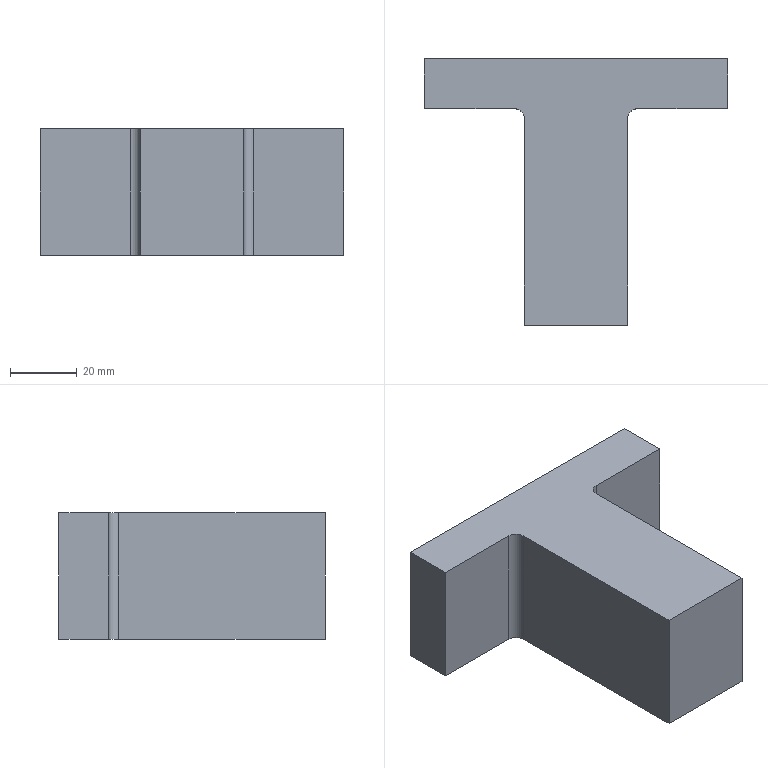Part | SolidWorks | features Extrusion 1, Fillet 1, ICE 1 | 1 solid | 12 faces | box 91 x 80 x 38 mm | volume 128587 mm3 | plane 10 | cylinder 2 | commonest cylinder face diameters 6 x2
STEP:
#1=CARTESIAN_POINT('',(45.5,25.,19.));
#2=VERTEX_POINT('',#1);
#3=CARTESIAN_POINT('',(45.5,40.,19.));
#4=VERTEX_POINT('',#3);
#5=CARTESIAN_POINT('',(45.5,-40.,19.));
#6=DIRECTION('',(0.,1.,0.));
#7=VECTOR('',#6,1000.);
#8=LINE('',#5,#7);
#9=EDGE_CURVE('',#2,#4,#8,.T.);
#10=ORIENTED_EDGE('',*,*,#9,.F.);
#11=CARTESIAN_POINT('',(45.5,25.,-19.));
#12=VERTEX_POINT('',#11);
#13=CARTESIAN_POINT('',(45.5,25.,-19.001));
#14=DIRECTION('',(0.,0.,1.));
#15=VECTOR('',#14,1000.);
#16=LINE('',#13,#15);
#17=EDGE_CURVE('',#12,#2,#16,.T.);
#18=ORIENTED_EDGE('',*,*,#17,.F.);
#19=CARTESIAN_POINT('',(45.5,40.,-19.));
#20=VERTEX_POINT('',#19);
#21=CARTESIAN_POINT('',(45.5,-40.,-19.));
#22=DIRECTION('',(0.,1.,0.));
#23=VECTOR('',#22,1000.);
#24=LINE('',#21,#23);
#25=EDGE_CURVE('',#12,#20,#24,.T.);
#26=ORIENTED_EDGE('',*,*,#25,.T.);
#27=CARTESIAN_POINT('',(45.5,40.,19.));
#28=DIRECTION('',(0.,0.,-1.));
#29=VECTOR('',#28,1000.);
#30=LINE('',#27,#29);
#31=EDGE_CURVE('',#4,#20,#30,.T.);
#32=ORIENTED_EDGE('',*,*,#31,.F.);
#33=EDGE_LOOP('',(#10,#18,#26,#32));
#34=FACE_OUTER_BOUND('',#33,.T.);
#35=CARTESIAN_POINT('',(45.5,-40.,19.));
#36=DIRECTION('',(-1.,0.,0.));
#37=DIRECTION('',(0.,0.,1.));
#38=AXIS2_PLACEMENT_3D('',#35,#36,#37);
#39=PLANE('',#38);
#40=ADVANCED_FACE('',(#34),#39,.F.);
#41=CARTESIAN_POINT('',(-45.5,40.,-19.));
#42=VERTEX_POINT('',#41);
#43=CARTESIAN_POINT('',(-45.5,40.,-19.));
#44=DIRECTION('',(-1.,0.,0.));
#45=VECTOR('',#44,1000.);
#46=LINE('',#43,#45);
#47=EDGE_CURVE('',#20,#42,#46,.T.);
#48=ORIENTED_EDGE('',*,*,#47,.T.);
#49=CARTESIAN_POINT('',(-45.5,40.,19.));
#50=VERTEX_POINT('',#49);
#51=CARTESIAN_POINT('',(-45.5,40.,19.));
#52=DIRECTION('',(0.,0.,-1.));
#53=VECTOR('',#52,1000.);
#54=LINE('',#51,#53);
#55=EDGE_CURVE('',#50,#42,#54,.T.);
#56=ORIENTED_EDGE('',*,*,#55,.F.);
#57=CARTESIAN_POINT('',(-45.5,40.,19.));
#58=DIRECTION('',(-1.,0.,0.));
#59=VECTOR('',#58,1000.);
#60=LINE('',#57,#59);
#61=EDGE_CURVE('',#4,#50,#60,.T.);
#62=ORIENTED_EDGE('',*,*,#61,.F.);
#63=ORIENTED_EDGE('',*,*,#31,.T.);
#64=EDGE_LOOP('',(#48,#56,#62,#63));
#65=FACE_OUTER_BOUND('',#64,.T.);
#66=CARTESIAN_POINT('',(-45.5,40.,19.));
#67=DIRECTION('',(0.,-1.,0.));
#68=DIRECTION('',(0.,0.,-1.));
#69=AXIS2_PLACEMENT_3D('',#66,#67,#68);
#70=PLANE('',#69);
#71=ADVANCED_FACE('',(#65),#70,.F.);
#72=CARTESIAN_POINT('',(-45.5,25.,-19.));
#73=VERTEX_POINT('',#72);
#74=CARTESIAN_POINT('',(-45.5,-40.,-19.));
#75=DIRECTION('',(0.,-1.,0.));
#76=VECTOR('',#75,1000.);
#77=LINE('',#74,#76);
#78=EDGE_CURVE('',#42,#73,#77,.T.);
#79=ORIENTED_EDGE('',*,*,#78,.T.);
#80=CARTESIAN_POINT('',(-45.5,25.,19.));
#81=VERTEX_POINT('',#80);
#82=CARTESIAN_POINT('',(-45.5,25.,-19.001));
#83=DIRECTION('',(0.,0.,1.));
#84=VECTOR('',#83,1000.);
#85=LINE('',#82,#84);
#86=EDGE_CURVE('',#73,#81,#85,.T.);
#87=ORIENTED_EDGE('',*,*,#86,.T.);
#88=CARTESIAN_POINT('',(-45.5,-40.,19.));
#89=DIRECTION('',(0.,-1.,0.));
#90=VECTOR('',#89,1000.);
#91=LINE('',#88,#90);
#92=EDGE_CURVE('',#50,#81,#91,.T.);
#93=ORIENTED_EDGE('',*,*,#92,.F.);
#94=ORIENTED_EDGE('',*,*,#55,.T.);
#95=EDGE_LOOP('',(#79,#87,#93,#94));
#96=FACE_OUTER_BOUND('',#95,.T.);
#97=CARTESIAN_POINT('',(-45.5,-40.,19.));
#98=DIRECTION('',(1.,0.,0.));
#99=DIRECTION('',(0.,0.,-1.));
#100=AXIS2_PLACEMENT_3D('',#97,#98,#99);
#101=PLANE('',#100);
#102=ADVANCED_FACE('',(#96),#101,.F.);
#103=CARTESIAN_POINT('',(-15.5,-40.,19.));
#104=VERTEX_POINT('',#103);
#105=CARTESIAN_POINT('',(15.5,-40.,19.));
#106=VERTEX_POINT('',#105);
#107=CARTESIAN_POINT('',(-45.5,-40.,19.));
#108=DIRECTION('',(1.,0.,0.));
#109=VECTOR('',#108,1000.);
#110=LINE('',#107,#109);
#111=EDGE_CURVE('',#104,#106,#110,.T.);
#112=ORIENTED_EDGE('',*,*,#111,.F.);
#113=CARTESIAN_POINT('',(-15.5,-40.,-19.));
#114=VERTEX_POINT('',#113);
#115=CARTESIAN_POINT('',(-15.5,-40.,-19.001));
#116=DIRECTION('',(0.,0.,1.));
#117=VECTOR('',#116,1000.);
#118=LINE('',#115,#117);
#119=EDGE_CURVE('',#114,#104,#118,.T.);
#120=ORIENTED_EDGE('',*,*,#119,.F.);
#121=CARTESIAN_POINT('',(15.5,-40.,-19.));
#122=VERTEX_POINT('',#121);
#123=CARTESIAN_POINT('',(-45.5,-40.,-19.));
#124=DIRECTION('',(1.,0.,0.));
#125=VECTOR('',#124,1000.);
#126=LINE('',#123,#125);
#127=EDGE_CURVE('',#114,#122,#126,.T.);
#128=ORIENTED_EDGE('',*,*,#127,.T.);
#129=CARTESIAN_POINT('',(15.5,-40.,-19.001));
#130=DIRECTION('',(0.,0.,1.));
#131=VECTOR('',#130,1000.);
#132=LINE('',#129,#131);
#133=EDGE_CURVE('',#122,#106,#132,.T.);
#134=ORIENTED_EDGE('',*,*,#133,.T.);
#135=EDGE_LOOP('',(#112,#120,#128,#134));
#136=FACE_OUTER_BOUND('',#135,.T.);
#137=CARTESIAN_POINT('',(-45.5,-40.,19.));
#138=DIRECTION('',(0.,1.,0.));
#139=DIRECTION('',(0.,0.,1.));
#140=AXIS2_PLACEMENT_3D('',#137,#138,#139);
#141=PLANE('',#140);
#142=ADVANCED_FACE('',(#136),#141,.F.);
#143=ORIENTED_EDGE('',*,*,#92,.T.);
#144=CARTESIAN_POINT('',(-18.5,25.,19.));
#145=VERTEX_POINT('',#144);
#146=CARTESIAN_POINT('',(-45.5,25.,19.));
#147=DIRECTION('',(-1.,0.,0.));
#148=VECTOR('',#147,1000.);
#149=LINE('',#146,#148);
#150=EDGE_CURVE('',#145,#81,#149,.T.);
#151=ORIENTED_EDGE('',*,*,#150,.F.);
#152=CARTESIAN_POINT('',(-15.5,22.,19.));
#153=VERTEX_POINT('',#152);
#154=CARTESIAN_POINT('',(-18.5,22.,19.));
#155=DIRECTION('',(0.,0.,-1.));
#156=DIRECTION('',(-1.,0.,0.));
#157=AXIS2_PLACEMENT_3D('',#154,#155,#156);
#158=CIRCLE('',#157,3.);
#159=EDGE_CURVE('',#145,#153,#158,.T.);
#160=ORIENTED_EDGE('',*,*,#159,.T.);
#161=CARTESIAN_POINT('',(-15.5,-40.,19.));
#162=DIRECTION('',(0.,1.,0.));
#163=VECTOR('',#162,1000.);
#164=LINE('',#161,#163);
#165=EDGE_CURVE('',#104,#153,#164,.T.);
#166=ORIENTED_EDGE('',*,*,#165,.F.);
#167=ORIENTED_EDGE('',*,*,#111,.T.);
#168=CARTESIAN_POINT('',(15.5,22.,19.));
#169=VERTEX_POINT('',#168);
#170=CARTESIAN_POINT('',(15.5,-40.,19.));
#171=DIRECTION('',(0.,-1.,0.));
#172=VECTOR('',#171,1000.);
#173=LINE('',#170,#172);
#174=EDGE_CURVE('',#169,#106,#173,.T.);
#175=ORIENTED_EDGE('',*,*,#174,.F.);
#176=CARTESIAN_POINT('',(18.5,25.,19.));
#177=VERTEX_POINT('',#176);
#178=CARTESIAN_POINT('',(18.5,22.,19.));
#179=DIRECTION('',(0.,0.,-1.));
#180=DIRECTION('',(-1.,0.,0.));
#181=AXIS2_PLACEMENT_3D('',#178,#179,#180);
#182=CIRCLE('',#181,3.);
#183=EDGE_CURVE('',#169,#177,#182,.T.);
#184=ORIENTED_EDGE('',*,*,#183,.T.);
#185=CARTESIAN_POINT('',(45.5,25.,19.));
#186=DIRECTION('',(-1.,0.,0.));
#187=VECTOR('',#186,1000.);
#188=LINE('',#185,#187);
#189=EDGE_CURVE('',#2,#177,#188,.T.);
#190=ORIENTED_EDGE('',*,*,#189,.F.);
#191=ORIENTED_EDGE('',*,*,#9,.T.);
#192=ORIENTED_EDGE('',*,*,#61,.T.);
#193=EDGE_LOOP('',(#143,#151,#160,#166,#167,#175,#184,#190,#191,#192));
#194=FACE_OUTER_BOUND('',#193,.T.);
#195=CARTESIAN_POINT('',(0.,0.,19.));
#196=DIRECTION('',(0.,0.,-1.));
#197=DIRECTION('',(-1.,0.,0.));
#198=AXIS2_PLACEMENT_3D('',#195,#196,#197);
#199=PLANE('',#198);
#200=ADVANCED_FACE('',(#194),#199,.F.);
#201=CARTESIAN_POINT('',(-15.5,22.,-19.));
#202=VERTEX_POINT('',#201);
#203=CARTESIAN_POINT('',(-15.5,-40.,-19.));
#204=DIRECTION('',(0.,1.,0.));
#205=VECTOR('',#204,1000.);
#206=LINE('',#203,#205);
#207=EDGE_CURVE('',#114,#202,#206,.T.);
#208=ORIENTED_EDGE('',*,*,#207,.T.);
#209=CARTESIAN_POINT('',(-18.5,25.,-19.));
#210=VERTEX_POINT('',#209);
#211=CARTESIAN_POINT('',(-18.5,22.,-19.));
#212=DIRECTION('',(0.,0.,1.));
#213=DIRECTION('',(-1.,0.,0.));
#214=AXIS2_PLACEMENT_3D('',#211,#212,#213);
#215=CIRCLE('',#214,3.);
#216=EDGE_CURVE('',#202,#210,#215,.T.);
#217=ORIENTED_EDGE('',*,*,#216,.T.);
#218=CARTESIAN_POINT('',(-45.5,25.,-19.));
#219=DIRECTION('',(-1.,0.,0.));
#220=VECTOR('',#219,1000.);
#221=LINE('',#218,#220);
#222=EDGE_CURVE('',#210,#73,#221,.T.);
#223=ORIENTED_EDGE('',*,*,#222,.T.);
#224=ORIENTED_EDGE('',*,*,#78,.F.);
#225=ORIENTED_EDGE('',*,*,#47,.F.);
#226=ORIENTED_EDGE('',*,*,#25,.F.);
#227=CARTESIAN_POINT('',(18.5,25.,-19.));
#228=VERTEX_POINT('',#227);
#229=CARTESIAN_POINT('',(45.5,25.,-19.));
#230=DIRECTION('',(-1.,0.,0.));
#231=VECTOR('',#230,1000.);
#232=LINE('',#229,#231);
#233=EDGE_CURVE('',#12,#228,#232,.T.);
#234=ORIENTED_EDGE('',*,*,#233,.T.);
#235=CARTESIAN_POINT('',(15.5,22.,-19.));
#236=VERTEX_POINT('',#235);
#237=CARTESIAN_POINT('',(18.5,22.,-19.));
#238=DIRECTION('',(0.,0.,1.));
#239=DIRECTION('',(-1.,0.,0.));
#240=AXIS2_PLACEMENT_3D('',#237,#238,#239);
#241=CIRCLE('',#240,3.);
#242=EDGE_CURVE('',#228,#236,#241,.T.);
#243=ORIENTED_EDGE('',*,*,#242,.T.);
#244=CARTESIAN_POINT('',(15.5,-40.,-19.));
#245=DIRECTION('',(0.,-1.,0.));
#246=VECTOR('',#245,1000.);
#247=LINE('',#244,#246);
#248=EDGE_CURVE('',#236,#122,#247,.T.);
#249=ORIENTED_EDGE('',*,*,#248,.T.);
#250=ORIENTED_EDGE('',*,*,#127,.F.);
#251=EDGE_LOOP('',(#208,#217,#223,#224,#225,#226,#234,#243,#249,#250));
#252=FACE_OUTER_BOUND('',#251,.T.);
#253=CARTESIAN_POINT('',(0.,0.,-19.));
#254=DIRECTION('',(0.,0.,-1.));
#255=DIRECTION('',(-1.,0.,0.));
#256=AXIS2_PLACEMENT_3D('',#253,#254,#255);
#257=PLANE('',#256);
#258=ADVANCED_FACE('',(#252),#257,.T.);
#259=ORIENTED_EDGE('',*,*,#248,.F.);
#260=CARTESIAN_POINT('',(15.5,22.,19.));
#261=DIRECTION('',(0.,0.,1.));
#262=VECTOR('',#261,1000.);
#263=LINE('',#260,#262);
#264=EDGE_CURVE('',#236,#169,#263,.T.);
#265=ORIENTED_EDGE('',*,*,#264,.T.);
#266=ORIENTED_EDGE('',*,*,#174,.T.);
#267=ORIENTED_EDGE('',*,*,#133,.F.);
#268=EDGE_LOOP('',(#259,#265,#266,#267));
#269=FACE_OUTER_BOUND('',#268,.T.);
#270=CARTESIAN_POINT('',(15.5,-40.,-19.001));
#271=DIRECTION('',(-1.,0.,0.));
#272=DIRECTION('',(0.,0.,1.));
#273=AXIS2_PLACEMENT_3D('',#270,#271,#272);
#274=PLANE('',#273);
#275=ADVANCED_FACE('',(#269),#274,.F.);
#276=ORIENTED_EDGE('',*,*,#189,.T.);
#277=CARTESIAN_POINT('',(18.5,25.,-19.));
#278=DIRECTION('',(0.,0.,-1.));
#279=VECTOR('',#278,1000.);
#280=LINE('',#277,#279);
#281=EDGE_CURVE('',#177,#228,#280,.T.);
#282=ORIENTED_EDGE('',*,*,#281,.T.);
#283=ORIENTED_EDGE('',*,*,#233,.F.);
#284=ORIENTED_EDGE('',*,*,#17,.T.);
#285=EDGE_LOOP('',(#276,#282,#283,#284));
#286=FACE_OUTER_BOUND('',#285,.T.);
#287=CARTESIAN_POINT('',(45.5,25.,-19.001));
#288=DIRECTION('',(0.,1.,0.));
#289=DIRECTION('',(-1.,0.,0.));
#290=AXIS2_PLACEMENT_3D('',#287,#288,#289);
#291=PLANE('',#290);
#292=ADVANCED_FACE('',(#286),#291,.F.);
#293=ORIENTED_EDGE('',*,*,#222,.F.);
#294=CARTESIAN_POINT('',(-18.5,25.,19.));
#295=DIRECTION('',(0.,0.,1.));
#296=VECTOR('',#295,1000.);
#297=LINE('',#294,#296);
#298=EDGE_CURVE('',#210,#145,#297,.T.);
#299=ORIENTED_EDGE('',*,*,#298,.T.);
#300=ORIENTED_EDGE('',*,*,#150,.T.);
#301=ORIENTED_EDGE('',*,*,#86,.F.);
#302=EDGE_LOOP('',(#293,#299,#300,#301));
#303=FACE_OUTER_BOUND('',#302,.T.);
#304=CARTESIAN_POINT('',(-45.5,25.,-19.001));
#305=DIRECTION('',(0.,1.,0.));
#306=DIRECTION('',(0.,0.,1.));
#307=AXIS2_PLACEMENT_3D('',#304,#305,#306);
#308=PLANE('',#307);
#309=ADVANCED_FACE('',(#303),#308,.F.);
#310=ORIENTED_EDGE('',*,*,#165,.T.);
#311=CARTESIAN_POINT('',(-15.5,22.,-19.));
#312=DIRECTION('',(0.,0.,-1.));
#313=VECTOR('',#312,1000.);
#314=LINE('',#311,#313);
#315=EDGE_CURVE('',#153,#202,#314,.T.);
#316=ORIENTED_EDGE('',*,*,#315,.T.);
#317=ORIENTED_EDGE('',*,*,#207,.F.);
#318=ORIENTED_EDGE('',*,*,#119,.T.);
#319=EDGE_LOOP('',(#310,#316,#317,#318));
#320=FACE_OUTER_BOUND('',#319,.T.);
#321=CARTESIAN_POINT('',(-15.5,-40.,-19.001));
#322=DIRECTION('',(1.,0.,0.));
#323=DIRECTION('',(0.,0.,-1.));
#324=AXIS2_PLACEMENT_3D('',#321,#322,#323);
#325=PLANE('',#324);
#326=ADVANCED_FACE('',(#320),#325,.F.);
#327=ORIENTED_EDGE('',*,*,#242,.F.);
#328=ORIENTED_EDGE('',*,*,#281,.F.);
#329=ORIENTED_EDGE('',*,*,#183,.F.);
#330=ORIENTED_EDGE('',*,*,#264,.F.);
#331=EDGE_LOOP('',(#327,#328,#329,#330));
#332=FACE_OUTER_BOUND('',#331,.T.);
#333=CARTESIAN_POINT('',(18.5,22.,-19.001));
#334=DIRECTION('',(0.,0.,-1.));
#335=DIRECTION('',(-1.,0.,0.));
#336=AXIS2_PLACEMENT_3D('',#333,#334,#335);
#337=CYLINDRICAL_SURFACE('',#336,3.);
#338=ADVANCED_FACE('',(#332),#337,.F.);
#339=ORIENTED_EDGE('',*,*,#216,.F.);
#340=ORIENTED_EDGE('',*,*,#315,.F.);
#341=ORIENTED_EDGE('',*,*,#159,.F.);
#342=ORIENTED_EDGE('',*,*,#298,.F.);
#343=EDGE_LOOP('',(#339,#340,#341,#342));
#344=FACE_OUTER_BOUND('',#343,.T.);
#345=CARTESIAN_POINT('',(-18.5,22.,-19.001));
#346=DIRECTION('',(0.,0.,-1.));
#347=DIRECTION('',(-1.,0.,0.));
#348=AXIS2_PLACEMENT_3D('',#345,#346,#347);
#349=CYLINDRICAL_SURFACE('',#348,3.);
#350=ADVANCED_FACE('',(#344),#349,.F.);
#351=CLOSED_SHELL('',(#40,#71,#102,#142,#200,#258,#275,#292,#309,#326,#338,#350));
#352=MANIFOLD_SOLID_BREP('',#351);
#353=CARTESIAN_POINT('',(0.,0.,0.));
#354=DIRECTION('',(0.,0.,1.));
#355=DIRECTION('',(1.,0.,0.));
#356=AXIS2_PLACEMENT_3D('',#353,#354,#355);
#357=(LENGTH_UNIT()NAMED_UNIT(*)SI_UNIT(.MILLI.,.METRE.));
#358=UNCERTAINTY_MEASURE_WITH_UNIT(LENGTH_MEASURE(0.00001),#357,'','');
#359=(NAMED_UNIT(*)PLANE_ANGLE_UNIT()SI_UNIT($,.RADIAN.));
#360=(NAMED_UNIT(*)SI_UNIT($,.STERADIAN.)SOLID_ANGLE_UNIT());
#361=(GEOMETRIC_REPRESENTATION_CONTEXT(3)GLOBAL_UNCERTAINTY_ASSIGNED_CONTEXT((#358))GLOBAL_UNIT_ASSIGNED_CONTEXT((#357,#359,#360))REPRESENTATION_CONTEXT('',''));
#362=ADVANCED_BREP_SHAPE_REPRESENTATION('',(#352,#356),#361);